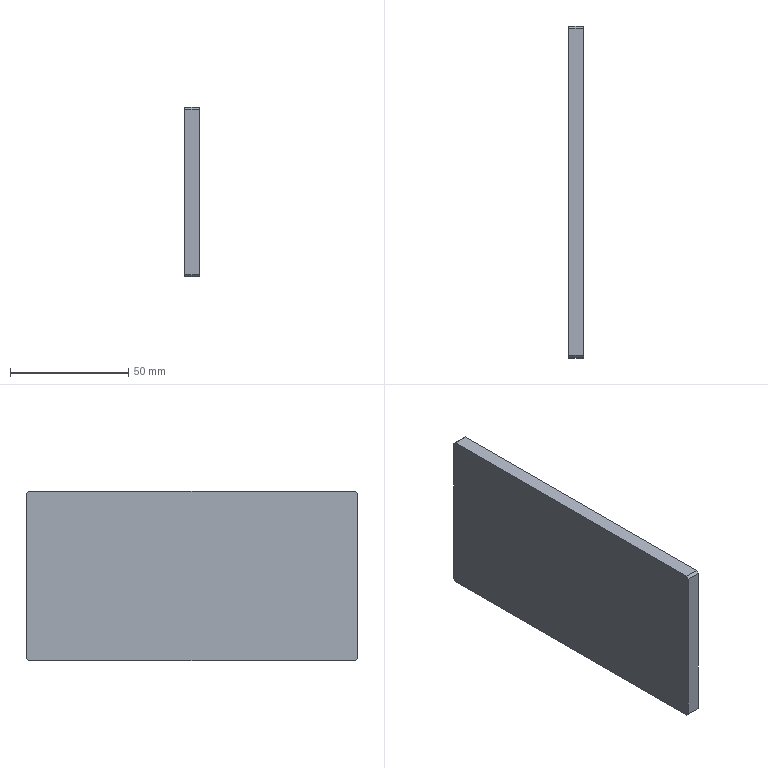Part | STEP file | 复件 FHB175-008^FHB175S-PRW-P40(马达RightUpper折-400W伺服电机) | 1 solid | 10 faces | box 6 x 140.5 x 72 mm | volume 60684 mm3 | plane 10
STEP:
#1=CARTESIAN_POINT('',(-37.,-157.,-59.));
#2=VERTEX_POINT('',#1);
#3=CARTESIAN_POINT('',(-37.,-158.,-58.));
#4=VERTEX_POINT('',#3);
#5=CARTESIAN_POINT('',(-37.,-158.,-58.));
#6=DIRECTION('',(0.,-0.7071,0.7071));
#7=VECTOR('',#6,1000.);
#8=LINE('',#5,#7);
#9=EDGE_CURVE('',#2,#4,#8,.T.);
#10=ORIENTED_EDGE('',*,*,#9,.T.);
#11=CARTESIAN_POINT('',(-37.,-158.,12.));
#12=VERTEX_POINT('',#11);
#13=CARTESIAN_POINT('',(-37.,-158.,0.));
#14=DIRECTION('',(0.,0.,-1.));
#15=VECTOR('',#14,1000.);
#16=LINE('',#13,#15);
#17=EDGE_CURVE('',#12,#4,#16,.T.);
#18=ORIENTED_EDGE('',*,*,#17,.F.);
#19=CARTESIAN_POINT('',(-37.,-157.,13.));
#20=VERTEX_POINT('',#19);
#21=CARTESIAN_POINT('',(-37.,-157.,13.));
#22=DIRECTION('',(0.,0.7071,0.7071));
#23=VECTOR('',#22,1000.);
#24=LINE('',#21,#23);
#25=EDGE_CURVE('',#12,#20,#24,.T.);
#26=ORIENTED_EDGE('',*,*,#25,.T.);
#27=CARTESIAN_POINT('',(-37.,-18.5,13.));
#28=VERTEX_POINT('',#27);
#29=CARTESIAN_POINT('',(-37.,0.,13.));
#30=DIRECTION('',(0.,-1.,0.));
#31=VECTOR('',#30,1000.);
#32=LINE('',#29,#31);
#33=EDGE_CURVE('',#28,#20,#32,.T.);
#34=ORIENTED_EDGE('',*,*,#33,.F.);
#35=CARTESIAN_POINT('',(-37.,-17.5,12.));
#36=VERTEX_POINT('',#35);
#37=CARTESIAN_POINT('',(-37.,-17.5,12.));
#38=DIRECTION('',(0.,0.7071,-0.7071));
#39=VECTOR('',#38,1000.);
#40=LINE('',#37,#39);
#41=EDGE_CURVE('',#28,#36,#40,.T.);
#42=ORIENTED_EDGE('',*,*,#41,.T.);
#43=CARTESIAN_POINT('',(-37.,-17.5,-58.));
#44=VERTEX_POINT('',#43);
#45=CARTESIAN_POINT('',(-37.,-17.5,0.));
#46=DIRECTION('',(0.,0.,1.));
#47=VECTOR('',#46,1000.);
#48=LINE('',#45,#47);
#49=EDGE_CURVE('',#44,#36,#48,.T.);
#50=ORIENTED_EDGE('',*,*,#49,.F.);
#51=CARTESIAN_POINT('',(-37.,-18.5,-59.));
#52=VERTEX_POINT('',#51);
#53=CARTESIAN_POINT('',(-37.,-18.5,-59.));
#54=DIRECTION('',(0.,-0.7071,-0.7071));
#55=VECTOR('',#54,1000.);
#56=LINE('',#53,#55);
#57=EDGE_CURVE('',#44,#52,#56,.T.);
#58=ORIENTED_EDGE('',*,*,#57,.T.);
#59=CARTESIAN_POINT('',(-37.,0.,-59.));
#60=DIRECTION('',(0.,1.,0.));
#61=VECTOR('',#60,1000.);
#62=LINE('',#59,#61);
#63=EDGE_CURVE('',#2,#52,#62,.T.);
#64=ORIENTED_EDGE('',*,*,#63,.F.);
#65=EDGE_LOOP('',(#10,#18,#26,#34,#42,#50,#58,#64));
#66=FACE_OUTER_BOUND('',#65,.T.);
#67=CARTESIAN_POINT('',(-37.,0.,0.));
#68=DIRECTION('',(1.,0.,0.));
#69=DIRECTION('',(0.,0.,-1.));
#70=AXIS2_PLACEMENT_3D('',#67,#68,#69);
#71=PLANE('',#70);
#72=ADVANCED_FACE('',(#66),#71,.F.);
#73=ORIENTED_EDGE('',*,*,#63,.T.);
#74=CARTESIAN_POINT('',(-31.,-18.5,-59.));
#75=VERTEX_POINT('',#74);
#76=CARTESIAN_POINT('',(-37.,-18.5,-59.));
#77=DIRECTION('',(1.,0.,0.));
#78=VECTOR('',#77,1000.);
#79=LINE('',#76,#78);
#80=EDGE_CURVE('',#52,#75,#79,.T.);
#81=ORIENTED_EDGE('',*,*,#80,.T.);
#82=CARTESIAN_POINT('',(-31.,-157.,-59.));
#83=VERTEX_POINT('',#82);
#84=CARTESIAN_POINT('',(-31.,-158.,-59.));
#85=DIRECTION('',(0.,-1.,0.));
#86=VECTOR('',#85,1000.);
#87=LINE('',#84,#86);
#88=EDGE_CURVE('',#75,#83,#87,.T.);
#89=ORIENTED_EDGE('',*,*,#88,.T.);
#90=CARTESIAN_POINT('',(-37.,-157.,-59.));
#91=DIRECTION('',(-1.,0.,0.));
#92=VECTOR('',#91,1000.);
#93=LINE('',#90,#92);
#94=EDGE_CURVE('',#83,#2,#93,.T.);
#95=ORIENTED_EDGE('',*,*,#94,.T.);
#96=EDGE_LOOP('',(#73,#81,#89,#95));
#97=FACE_OUTER_BOUND('',#96,.T.);
#98=CARTESIAN_POINT('',(-37.,-158.,-59.));
#99=DIRECTION('',(0.,0.,-1.));
#100=DIRECTION('',(-1.,0.,0.));
#101=AXIS2_PLACEMENT_3D('',#98,#99,#100);
#102=PLANE('',#101);
#103=ADVANCED_FACE('',(#97),#102,.T.);
#104=CARTESIAN_POINT('',(-31.,-158.,-58.));
#105=VERTEX_POINT('',#104);
#106=CARTESIAN_POINT('',(-31.,-158.,12.));
#107=VERTEX_POINT('',#106);
#108=CARTESIAN_POINT('',(-31.,-158.,13.));
#109=DIRECTION('',(0.,0.,1.));
#110=VECTOR('',#109,1000.);
#111=LINE('',#108,#110);
#112=EDGE_CURVE('',#105,#107,#111,.T.);
#113=ORIENTED_EDGE('',*,*,#112,.T.);
#114=CARTESIAN_POINT('',(-37.,-158.,12.));
#115=DIRECTION('',(-1.,0.,0.));
#116=VECTOR('',#115,1000.);
#117=LINE('',#114,#116);
#118=EDGE_CURVE('',#107,#12,#117,.T.);
#119=ORIENTED_EDGE('',*,*,#118,.T.);
#120=ORIENTED_EDGE('',*,*,#17,.T.);
#121=CARTESIAN_POINT('',(-37.,-158.,-58.));
#122=DIRECTION('',(1.,0.,0.));
#123=VECTOR('',#122,1000.);
#124=LINE('',#121,#123);
#125=EDGE_CURVE('',#4,#105,#124,.T.);
#126=ORIENTED_EDGE('',*,*,#125,.T.);
#127=EDGE_LOOP('',(#113,#119,#120,#126));
#128=FACE_OUTER_BOUND('',#127,.T.);
#129=CARTESIAN_POINT('',(-37.,-158.,13.));
#130=DIRECTION('',(0.,-1.,0.));
#131=DIRECTION('',(0.,0.,-1.));
#132=AXIS2_PLACEMENT_3D('',#129,#130,#131);
#133=PLANE('',#132);
#134=ADVANCED_FACE('',(#128),#133,.T.);
#135=CARTESIAN_POINT('',(-31.,-157.,13.));
#136=VERTEX_POINT('',#135);
#137=CARTESIAN_POINT('',(-31.,-18.5,13.));
#138=VERTEX_POINT('',#137);
#139=CARTESIAN_POINT('',(-31.,-17.5,13.));
#140=DIRECTION('',(0.,1.,0.));
#141=VECTOR('',#140,1000.);
#142=LINE('',#139,#141);
#143=EDGE_CURVE('',#136,#138,#142,.T.);
#144=ORIENTED_EDGE('',*,*,#143,.T.);
#145=CARTESIAN_POINT('',(-37.,-18.5,13.));
#146=DIRECTION('',(-1.,0.,0.));
#147=VECTOR('',#146,1000.);
#148=LINE('',#145,#147);
#149=EDGE_CURVE('',#138,#28,#148,.T.);
#150=ORIENTED_EDGE('',*,*,#149,.T.);
#151=ORIENTED_EDGE('',*,*,#33,.T.);
#152=CARTESIAN_POINT('',(-37.,-157.,13.));
#153=DIRECTION('',(1.,0.,0.));
#154=VECTOR('',#153,1000.);
#155=LINE('',#152,#154);
#156=EDGE_CURVE('',#20,#136,#155,.T.);
#157=ORIENTED_EDGE('',*,*,#156,.T.);
#158=EDGE_LOOP('',(#144,#150,#151,#157));
#159=FACE_OUTER_BOUND('',#158,.T.);
#160=CARTESIAN_POINT('',(-37.,-17.5,13.));
#161=DIRECTION('',(0.,0.,1.));
#162=DIRECTION('',(1.,0.,0.));
#163=AXIS2_PLACEMENT_3D('',#160,#161,#162);
#164=PLANE('',#163);
#165=ADVANCED_FACE('',(#159),#164,.T.);
#166=ORIENTED_EDGE('',*,*,#49,.T.);
#167=CARTESIAN_POINT('',(-31.,-17.5,12.));
#168=VERTEX_POINT('',#167);
#169=CARTESIAN_POINT('',(-37.,-17.5,12.));
#170=DIRECTION('',(1.,0.,0.));
#171=VECTOR('',#170,1000.);
#172=LINE('',#169,#171);
#173=EDGE_CURVE('',#36,#168,#172,.T.);
#174=ORIENTED_EDGE('',*,*,#173,.T.);
#175=CARTESIAN_POINT('',(-31.,-17.5,-58.));
#176=VERTEX_POINT('',#175);
#177=CARTESIAN_POINT('',(-31.,-17.5,-59.));
#178=DIRECTION('',(0.,0.,-1.));
#179=VECTOR('',#178,1000.);
#180=LINE('',#177,#179);
#181=EDGE_CURVE('',#168,#176,#180,.T.);
#182=ORIENTED_EDGE('',*,*,#181,.T.);
#183=CARTESIAN_POINT('',(-37.,-17.5,-58.));
#184=DIRECTION('',(-1.,0.,0.));
#185=VECTOR('',#184,1000.);
#186=LINE('',#183,#185);
#187=EDGE_CURVE('',#176,#44,#186,.T.);
#188=ORIENTED_EDGE('',*,*,#187,.T.);
#189=EDGE_LOOP('',(#166,#174,#182,#188));
#190=FACE_OUTER_BOUND('',#189,.T.);
#191=CARTESIAN_POINT('',(-37.,-17.5,-59.));
#192=DIRECTION('',(0.,1.,0.));
#193=DIRECTION('',(0.,0.,1.));
#194=AXIS2_PLACEMENT_3D('',#191,#192,#193);
#195=PLANE('',#194);
#196=ADVANCED_FACE('',(#190),#195,.T.);
#197=ORIENTED_EDGE('',*,*,#187,.F.);
#198=CARTESIAN_POINT('',(-31.,-18.5,-59.));
#199=DIRECTION('',(0.,0.7071,0.7071));
#200=VECTOR('',#199,1000.);
#201=LINE('',#198,#200);
#202=EDGE_CURVE('',#75,#176,#201,.T.);
#203=ORIENTED_EDGE('',*,*,#202,.F.);
#204=ORIENTED_EDGE('',*,*,#80,.F.);
#205=ORIENTED_EDGE('',*,*,#57,.F.);
#206=EDGE_LOOP('',(#197,#203,#204,#205));
#207=FACE_OUTER_BOUND('',#206,.T.);
#208=CARTESIAN_POINT('',(-37.,-18.5,-59.));
#209=DIRECTION('',(0.,-0.7071,0.7071));
#210=DIRECTION('',(0.,-0.7071,-0.7071));
#211=AXIS2_PLACEMENT_3D('',#208,#209,#210);
#212=PLANE('',#211);
#213=ADVANCED_FACE('',(#207),#212,.F.);
#214=ORIENTED_EDGE('',*,*,#94,.F.);
#215=CARTESIAN_POINT('',(-31.,-158.,-58.));
#216=DIRECTION('',(0.,0.7071,-0.7071));
#217=VECTOR('',#216,1000.);
#218=LINE('',#215,#217);
#219=EDGE_CURVE('',#105,#83,#218,.T.);
#220=ORIENTED_EDGE('',*,*,#219,.F.);
#221=ORIENTED_EDGE('',*,*,#125,.F.);
#222=ORIENTED_EDGE('',*,*,#9,.F.);
#223=EDGE_LOOP('',(#214,#220,#221,#222));
#224=FACE_OUTER_BOUND('',#223,.T.);
#225=CARTESIAN_POINT('',(-37.,-158.,-58.));
#226=DIRECTION('',(0.,0.7071,0.7071));
#227=DIRECTION('',(0.,-0.7071,0.7071));
#228=AXIS2_PLACEMENT_3D('',#225,#226,#227);
#229=PLANE('',#228);
#230=ADVANCED_FACE('',(#224),#229,.F.);
#231=ORIENTED_EDGE('',*,*,#143,.F.);
#232=CARTESIAN_POINT('',(-31.,-157.,13.));
#233=DIRECTION('',(0.,-0.7071,-0.7071));
#234=VECTOR('',#233,1000.);
#235=LINE('',#232,#234);
#236=EDGE_CURVE('',#136,#107,#235,.T.);
#237=ORIENTED_EDGE('',*,*,#236,.T.);
#238=ORIENTED_EDGE('',*,*,#112,.F.);
#239=ORIENTED_EDGE('',*,*,#219,.T.);
#240=ORIENTED_EDGE('',*,*,#88,.F.);
#241=ORIENTED_EDGE('',*,*,#202,.T.);
#242=ORIENTED_EDGE('',*,*,#181,.F.);
#243=CARTESIAN_POINT('',(-31.,-17.5,12.));
#244=DIRECTION('',(0.,-0.7071,0.7071));
#245=VECTOR('',#244,1000.);
#246=LINE('',#243,#245);
#247=EDGE_CURVE('',#168,#138,#246,.T.);
#248=ORIENTED_EDGE('',*,*,#247,.T.);
#249=EDGE_LOOP('',(#231,#237,#238,#239,#240,#241,#242,#248));
#250=FACE_OUTER_BOUND('',#249,.T.);
#251=CARTESIAN_POINT('',(-31.,0.,0.));
#252=DIRECTION('',(1.,0.,0.));
#253=DIRECTION('',(0.,0.,-1.));
#254=AXIS2_PLACEMENT_3D('',#251,#252,#253);
#255=PLANE('',#254);
#256=ADVANCED_FACE('',(#250),#255,.T.);
#257=ORIENTED_EDGE('',*,*,#118,.F.);
#258=ORIENTED_EDGE('',*,*,#236,.F.);
#259=ORIENTED_EDGE('',*,*,#156,.F.);
#260=ORIENTED_EDGE('',*,*,#25,.F.);
#261=EDGE_LOOP('',(#257,#258,#259,#260));
#262=FACE_OUTER_BOUND('',#261,.T.);
#263=CARTESIAN_POINT('',(-37.,-157.,13.));
#264=DIRECTION('',(0.,0.7071,-0.7071));
#265=DIRECTION('',(0.,0.7071,0.7071));
#266=AXIS2_PLACEMENT_3D('',#263,#264,#265);
#267=PLANE('',#266);
#268=ADVANCED_FACE('',(#262),#267,.F.);
#269=ORIENTED_EDGE('',*,*,#149,.F.);
#270=ORIENTED_EDGE('',*,*,#247,.F.);
#271=ORIENTED_EDGE('',*,*,#173,.F.);
#272=ORIENTED_EDGE('',*,*,#41,.F.);
#273=EDGE_LOOP('',(#269,#270,#271,#272));
#274=FACE_OUTER_BOUND('',#273,.T.);
#275=CARTESIAN_POINT('',(-37.,-17.5,12.));
#276=DIRECTION('',(0.,-0.7071,-0.7071));
#277=DIRECTION('',(0.,0.7071,-0.7071));
#278=AXIS2_PLACEMENT_3D('',#275,#276,#277);
#279=PLANE('',#278);
#280=ADVANCED_FACE('',(#274),#279,.F.);
#281=CLOSED_SHELL('',(#72,#103,#134,#165,#196,#213,#230,#256,#268,#280));
#282=MANIFOLD_SOLID_BREP('',#281);
#283=CARTESIAN_POINT('',(0.,0.,0.));
#284=DIRECTION('',(0.,0.,1.));
#285=DIRECTION('',(1.,0.,0.));
#286=AXIS2_PLACEMENT_3D('',#283,#284,#285);
#287=(LENGTH_UNIT()NAMED_UNIT(*)SI_UNIT(.MILLI.,.METRE.));
#288=UNCERTAINTY_MEASURE_WITH_UNIT(LENGTH_MEASURE(0.00001),#287,'','');
#289=(NAMED_UNIT(*)PLANE_ANGLE_UNIT()SI_UNIT($,.RADIAN.));
#290=(NAMED_UNIT(*)SI_UNIT($,.STERADIAN.)SOLID_ANGLE_UNIT());
#291=(GEOMETRIC_REPRESENTATION_CONTEXT(3)GLOBAL_UNCERTAINTY_ASSIGNED_CONTEXT((#288))GLOBAL_UNIT_ASSIGNED_CONTEXT((#287,#289,#290))REPRESENTATION_CONTEXT('',''));
#292=ADVANCED_BREP_SHAPE_REPRESENTATION('',(#282,#286),#291);